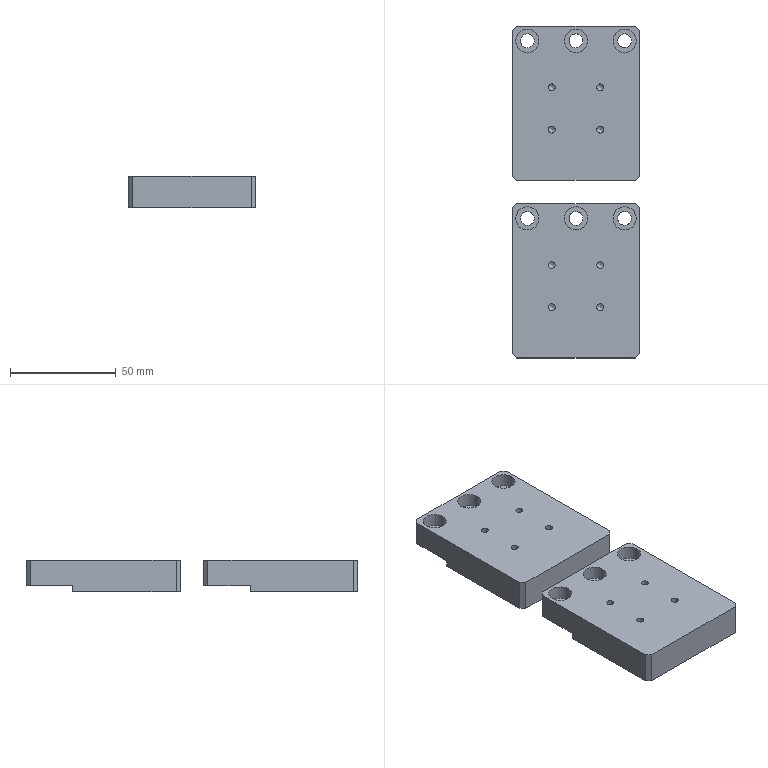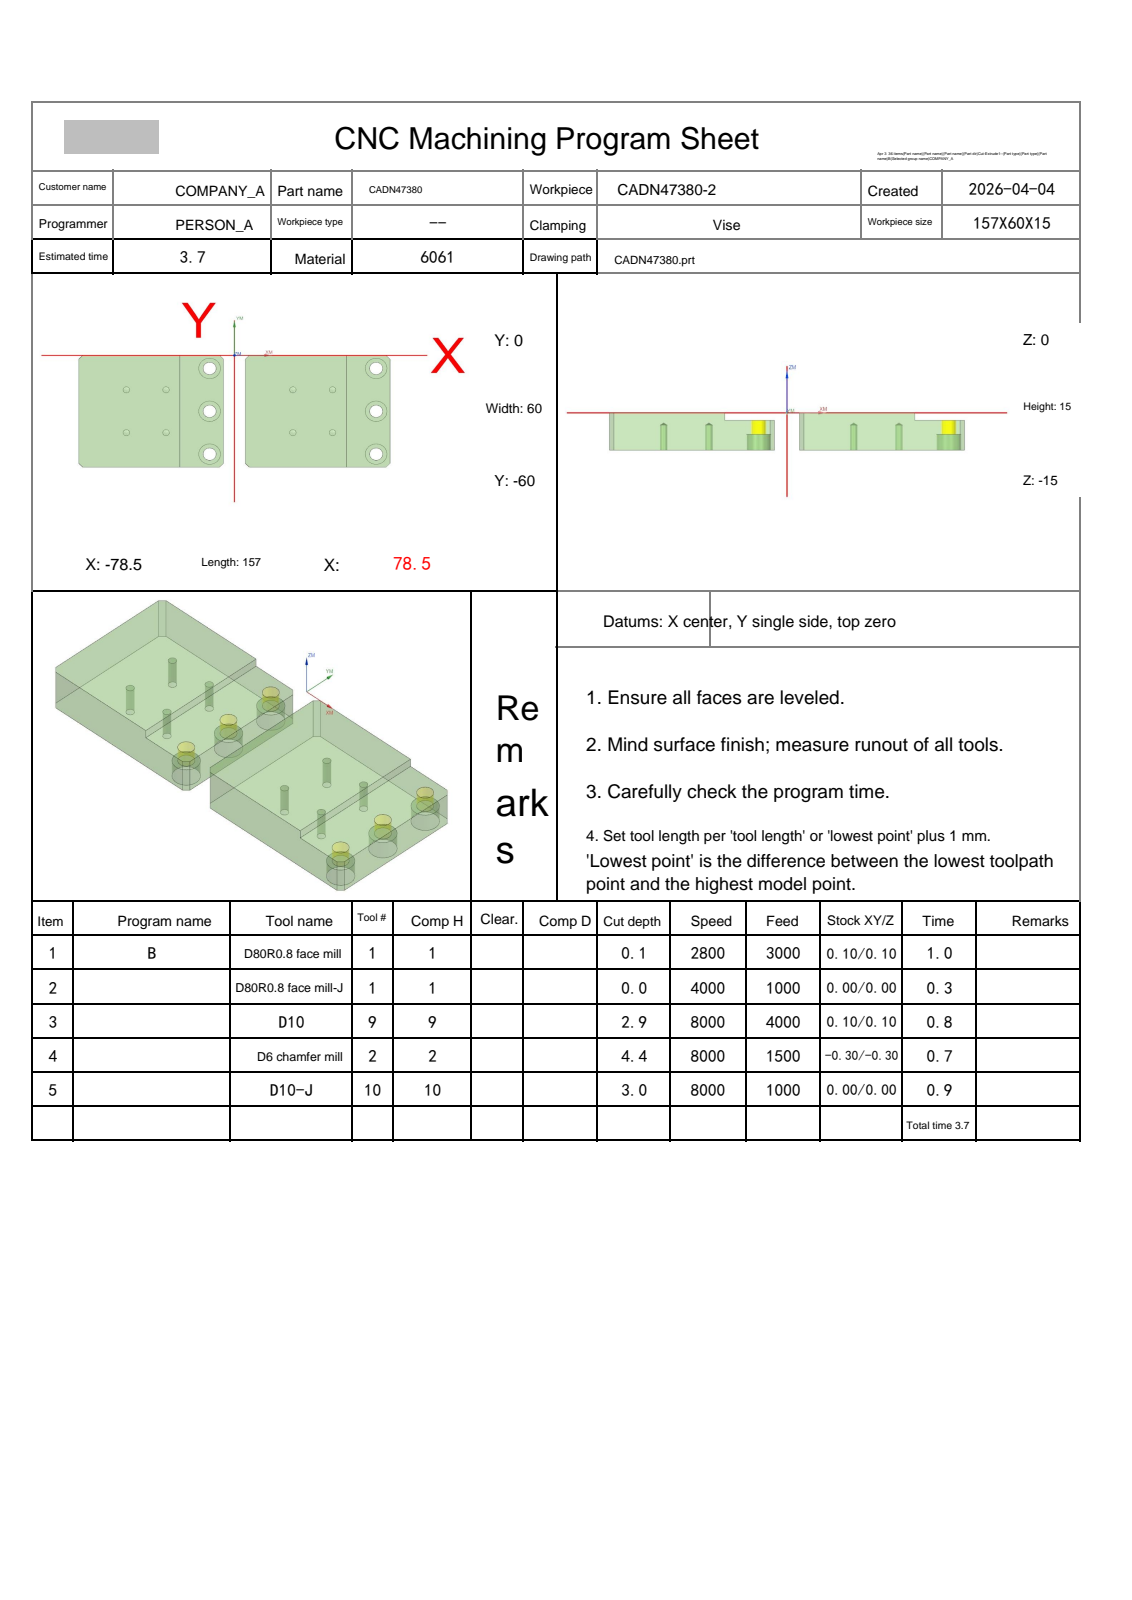NC program | NX | posted by the shop | part box 60 x 157 x 15 mm
Whole program:
%
O0001
(Machine time: 4.68 MIN)
(===Total Tool:4===)
(T1=D80R0.8 face mill D=80.  R=0.8  D-  H01 Z=0.    )
(T9=D10     D=10.  R=0.   D-  H09 Z=-2.9  )
(T2=D6 chamfer mill   D=6.   R=0.   D-  H02 Z=-4.4  )
(T10=D10-J  D=10.  R=0.   D10 H10 Z=-3.   )
G80 G90 G17 G49 G40
G91 G28 Z0
M01
N1 T01 M06
(D80R0.8 face mill  D=80. R=0.8 H=01 ce=0.10 di=0.10)
G00 G90 G54 X-130.597 Y-30. M03 S2800
G43 H01 Z20.
M08
Z6.011
G01 Z4.011 F3000.
X-118.597
X118.597
X130.597
Z6.011
G00 X-130.597
Z5.522
G01 Z3.522
X-118.597
X118.597
X130.597
Z5.522
G00 X-130.597
Z5.033
G01 Z3.033
X-118.597
X118.597
X130.597
Z5.033
G00 X-130.597
Z4.544
G01 Z2.544
X-118.597
X118.597
X130.597
Z4.544
G00 Z20.
X-130.597
Z4.056
G01 Z2.056
X-118.597
X118.597
X130.597
Z4.056
G00 Z20.
X-130.597
Z3.567
G01 Z1.567
X-118.597
X118.597
X130.597
Z3.567
G00 Z20.
X-130.597
Z3.078
G01 Z1.078
X-118.597
X118.597
X130.597
Z3.078
G00 Z20.
X-130.597
Z2.589
G01 Z.589
X-118.597
X118.597
X130.597
Z2.589
G00 Z20.
X-130.597
Z2.1
G01 Z.1
X-118.597
X118.597
X130.597
Z2.1
G00 Z20.
G91 G28 Z0.0
M05
M09
G91 G28 Z0.0
M01
N2 T01 M06
(D80R0.8 face mill-J  D=80. R=0.8 H=01 ce=0.00 di=0.00)
G00 G90 G54 X-130.499 Y-30. M03 S4000
G43 H01 Z20.
M08
Z2.
G01 Z0.0 F1000.
X-118.499
X118.499
X130.499
Z2.
G00 Z20.
G91 G28 Z0.0
M05
M09
G91 G28 Z0.0
M01
N3 T09 M06
(D10  D=10. R=0. H=09 ce=0.10 di=0.10)
G00 G90 G54 X-2.4 Y-66.214 M03 S8000
G43 H09 Z14.5
M08
Z.92
G01 Z-.58 F4000.
Y-61.83
Y1.416
G03 X-2.692 Y2.122 I-1. J-.001
G01 X-5.178 Y4.607
G03 X-5.884 Y4.9 I-.707 J-.707
G01 X-6.401
G03 X-7.4 Y3.901 I.001 J-1.
G01 Y-63.901
G02 X-8.399 Y-64.9 I-1. J.001
G01 X-13.901
G02 X-14.9 Y-63.901 I.001 J1.
G01 Y4.044
G03 X-15.746 Y5.032 I-1. J-.001
G01 X-21.246 Y5.888
X-21.4 Y5.9
G03 X-22.4 Y4.9 I0.0 J-1.
G01 Y-64.9
Y-68.1
Z.92
G00 X-2.4 Y-66.214
Z.34
G01 Z-1.16
Y-61.83
Y1.416
G03 X-2.692 Y2.122 I-1. J-.001
G01 X-5.178 Y4.607
G03 X-5.884 Y4.9 I-.707 J-.707
G01 X-6.401
G03 X-7.4 Y3.901 I.001 J-1.
G01 Y-63.901
G02 X-8.399 Y-64.9 I-1. J.001
G01 X-13.901
G02 X-14.9 Y-63.901 I.001 J1.
G01 Y4.044
G03 X-15.746 Y5.032 I-1. J-.001
G01 X-21.246 Y5.888
X-21.4 Y5.9
G03 X-22.4 Y4.9 I0.0 J-1.
G01 Y-64.9
Y-68.1
Z.34
G00 X-2.4 Y-66.214
Z-.24
G01 Z-1.74
Y-61.83
Y1.416
G03 X-2.692 Y2.122 I-1. J-.001
G01 X-5.178 Y4.607
G03 X-5.884 Y4.9 I-.707 J-.707
G01 X-6.401
G03 X-7.4 Y3.901 I.001 J-1.
G01 Y-63.901
G02 X-8.399 Y-64.9 I-1. J.001
G01 X-13.901
G02 X-14.9 Y-63.901 I.001 J1.
G01 Y4.044
G03 X-15.746 Y5.032 I-1. J-.001
G01 X-21.246 Y5.888
X-21.4 Y5.9
G03 X-22.4 Y4.9 I0.0 J-1.
G01 Y-64.9
Y-68.1
Z-.24
G00 X-2.4 Y-66.214
Z-.82
G01 Z-2.32
Y-61.83
Y1.416
G03 X-2.692 Y2.122 I-1. J-.001
G01 X-5.178 Y4.607
G03 X-5.884 Y4.9 I-.707 J-.707
G01 X-6.401
G03 X-7.4 Y3.901 I.001 J-1.
G01 Y-63.901
G02 X-8.399 Y-64.9 I-1. J.001
G01 X-13.901
G02 X-14.9 Y-63.901 I.001 J1.
G01 Y4.044
G03 X-15.746 Y5.032 I-1. J-.001
G01 X-21.246 Y5.888
X-21.4 Y5.9
G03 X-22.4 Y4.9 I0.0 J-1.
G01 Y-64.9
Y-68.1
Z-.82
G00 X-2.4 Y-66.214
Z-1.4
G01 Z-2.9
Y-61.83
Y1.416
G03 X-2.692 Y2.122 I-1. J-.001
G01 X-5.178 Y4.607
G03 X-5.884 Y4.9 I-.707 J-.707
G01 X-6.401
G03 X-7.4 Y3.901 I.001 J-1.
G01 Y-63.901
G02 X-8.399 Y-64.9 I-1. J.001
G01 X-13.901
G02 X-14.9 Y-63.901 I.001 J1.
G01 Y4.044
G03 X-15.746 Y5.032 I-1. J-.001
G01 X-21.246 Y5.888
X-21.4 Y5.9
G03 X-22.4 Y4.9 I0.0 J-1.
G01 Y-64.9
Y-68.1
Z-1.4
G00 Z3.
X81.6 Y-66.214
Z.92
G01 Z-.58
Y-61.83
Y1.416
G03 X81.308 Y2.122 I-1. J-.001
G01 X78.822 Y4.607
G03 X78.116 Y4.9 I-.707 J-.707
G01 X77.599
G03 X76.6 Y3.901 I.001 J-1.
G01 Y-63.901
G02 X75.601 Y-64.9 I-1. J.001
G01 X70.099
G02 X69.1 Y-63.901 I.001 J1.
G01 Y4.044
G03 X68.254 Y5.032 I-1. J-.001
G01 X62.754 Y5.888
X62.6 Y5.9
G03 X61.6 Y4.9 I0.0 J-1.
G01 Y-64.9
Y-68.1
Z.92
G00 X81.6 Y-66.214
Z.34
G01 Z-1.16
Y-61.83
Y1.416
G03 X81.308 Y2.122 I-1. J-.001
G01 X78.822 Y4.607
G03 X78.116 Y4.9 I-.707 J-.707
G01 X77.599
G03 X76.6 Y3.901 I.001 J-1.
G01 Y-63.901
G02 X75.601 Y-64.9 I-1. J.001
G01 X70.099
G02 X69.1 Y-63.901 I.001 J1.
G01 Y4.044
G03 X68.254 Y5.032 I-1. J-.001
G01 X62.754 Y5.888
X62.6 Y5.9
G03 X61.6 Y4.9 I0.0 J-1.
G01 Y-64.9
Y-68.1
Z.34
G00 X81.6 Y-66.214
Z-.24
G01 Z-1.74
Y-61.83
Y1.416
G03 X81.308 Y2.122 I-1. J-.001
G01 X78.822 Y4.607
G03 X78.116 Y4.9 I-.707 J-.707
G01 X77.599
G03 X76.6 Y3.901 I.001 J-1.
G01 Y-63.901
G02 X75.601 Y-64.9 I-1. J.001
G01 X70.099
G02 X69.1 Y-63.901 I.001 J1.
G01 Y4.044
G03 X68.254 Y5.032 I-1. J-.001
G01 X62.754 Y5.888
X62.6 Y5.9
G03 X61.6 Y4.9 I0.0 J-1.
G01 Y-64.9
Y-68.1
Z-.24
G00 X81.6 Y-66.214
Z-.82
G01 Z-2.32
Y-61.83
Y1.416
G03 X81.308 Y2.122 I-1. J-.001
G01 X78.822 Y4.607
G03 X78.116 Y4.9 I-.707 J-.707
G01 X77.599
G03 X76.6 Y3.901 I.001 J-1.
G01 Y-63.901
G02 X75.601 Y-64.9 I-1. J.001
G01 X70.099
G02 X69.1 Y-63.901 I.001 J1.
G01 Y4.044
G03 X68.254 Y5.032 I-1. J-.001
G01 X62.754 Y5.888
X62.6 Y5.9
G03 X61.6 Y4.9 I0.0 J-1.
G01 Y-64.9
Y-68.1
Z-.82
G00 X81.6 Y-66.214
Z-1.4
G01 Z-2.9
Y-61.83
Y1.416
G03 X81.308 Y2.122 I-1. J-.001
G01 X78.822 Y4.607
G03 X78.116 Y4.9 I-.707 J-.707
G01 X77.599
G03 X76.6 Y3.901 I.001 J-1.
G01 Y-63.901
G02 X75.601 Y-64.9 I-1. J.001
G01 X70.099
G02 X69.1 Y-63.901 I.001 J1.
G01 Y4.044
G03 X68.254 Y5.032 I-1. J-.001
G01 X62.754 Y5.888
X62.6 Y5.9
G03 X61.6 Y4.9 I0.0 J-1.
G01 Y-64.9
Y-68.1
Z-1.4
G00 Z14.5
G91 G28 Z0.0
M05
M09
G91 G28 Z0.0
M01
N4 T02 M06
(D6 chamfer mill  D=6. R=0. H=02 ce=-0.30 di=-0.80)
G00 G90 G54 X-11.413 Y-52.493 M03 S8000
G43 H02 Z20.
M08
Z-3.9
G01 Z-4.4 F1200.
X-11. Y-52.3
G03 X-12.5 Y-50.8 I-1.5 J0.0
X-14.7 Y-53. I0.0 J-2.2
X-12.5 Y-55.2 I2.2 J0.0
X-10.3 Y-53. I0.0 J2.2
X-12.5 Y-50.8 I-2.2 J0.0
X-14. Y-52.3 I0.0 J-1.5
G01 X-13.587 Y-52.493
Z-3.9
G00 Z20.
X-11.413 Y-29.493
Z-3.9
G01 Z-4.4
X-11. Y-29.3
G03 X-12.5 Y-27.8 I-1.5 J0.0
X-14.7 Y-30. I0.0 J-2.2
X-12.5 Y-32.2 I2.2 J0.0
X-10.3 Y-30. I0.0 J2.2
X-12.5 Y-27.8 I-2.2 J0.0
X-14. Y-29.3 I0.0 J-1.5
G01 X-13.587 Y-29.493
Z-3.9
G00 Z20.
X-11.413 Y-6.493
Z-3.9
G01 Z-4.4
X-11. Y-6.3
G03 X-12.5 Y-4.8 I-1.5 J0.0
X-14.7 Y-7. I0.0 J-2.2
X-12.5 Y-9.2 I2.2 J0.0
X-10.3 Y-7. I0.0 J2.2
X-12.5 Y-4.8 I-2.2 J0.0
X-14. Y-6.3 I0.0 J-1.5
G01 X-13.587 Y-6.493
Z-3.9
G00 Z20.
X72.587
Z-3.9
G01 Z-4.4
X73. Y-6.3
G03 X71.5 Y-4.8 I-1.5 J0.0
X69.3 Y-7. I0.0 J-2.2
X71.5 Y-9.2 I2.2 J0.0
X73.7 Y-7. I0.0 J2.2
X71.5 Y-4.8 I-2.2 J0.0
X70. Y-6.3 I0.0 J-1.5
G01 X70.413 Y-6.493
Z-3.9
G00 Z20.
X72.587 Y-29.493
Z-3.9
G01 Z-4.4
X73. Y-29.3
G03 X71.5 Y-27.8 I-1.5 J0.0
X69.3 Y-30. I0.0 J-2.2
X71.5 Y-32.2 I2.2 J0.0
X73.7 Y-30. I0.0 J2.2
X71.5 Y-27.8 I-2.2 J0.0
X70. Y-29.3 I0.0 J-1.5
G01 X70.413 Y-29.493
Z-3.9
G00 Z20.
X72.587 Y-52.493
Z-3.9
G01 Z-4.4
X73. Y-52.3
G03 X71.5 Y-50.8 I-1.5 J0.0
X69.3 Y-53. I0.0 J-2.2
X71.5 Y-55.2 I2.2 J0.0
X73.7 Y-53. I0.0 J2.2
X71.5 Y-50.8 I-2.2 J0.0
X70. Y-52.3 I0.0 J-1.5
G01 X70.413 Y-52.493
Z-3.9
G00 Z20.
G00 G90 X57.627 Y-29.614 M03 S8000
Z20.
Z.272
G01 Z-1.2 F1350.
G03 X57.427 Y-29.9 I1.532 J-1.286
G01 X57.397 Y-29.946
X57.4 Y-30.
Y-60. F1500.
G02 X56.5 Y-60.9 I-.9 J0.0
G01 X7.5
X7.267 Y-60.869
X7.05 Y-60.779
X6.864 Y-60.636
X4.864 Y-58.636
X4.721 Y-58.45
X4.631 Y-58.233
X4.6 Y-58.
Y-2.
X4.631 Y-1.767
X4.721 Y-1.55
X4.864 Y-1.364
X6.864 Y.636
X7.05 Y.779
X7.267 Y.869
X7.5 Y.9
X56.5
G02 X57.4 Y0.0 I0.0 J-.9
G01 Y-30.
X57.397 Y-30.054
X57.427 Y-30.1
G03 X57.627 Y-30.386 I1.732 J1.
G01 Z.272
G00 Z10.
X-26.373 Y-29.614
Z.272
G01 Z-1.2 F1350.
G03 X-26.573 Y-29.9 I1.532 J-1.286
G01 X-26.603 Y-29.946
X-26.6 Y-30.
Y-60. F1500.
G02 X-27.5 Y-60.9 I-.9 J0.0
G01 X-76.5
X-76.733 Y-60.869
X-76.95 Y-60.779
X-77.136 Y-60.636
X-79.136 Y-58.636
X-79.279 Y-58.45
X-79.369 Y-58.233
X-79.4 Y-58.
Y-2.
X-79.369 Y-1.767
X-79.279 Y-1.55
X-79.136 Y-1.364
X-77.136 Y.636
X-76.95 Y.779
X-76.733 Y.869
X-76.5 Y.9
X-27.5
G02 X-26.6 Y0.0 I0.0 J-.9
G01 Y-30.
X-26.603 Y-30.054
X-26.573 Y-30.1
G03 X-26.373 Y-30.386 I1.732 J1.
G01 Z.272
G00 Z10.
X-24.452 Y.968
Z-1.8
G01 Z-4.2 F1350.
X-24.366 Y.908
X-24.336 Y.9
X-7.5 F1500.
X-7.267 Y.869
X-7.05 Y.779
X-6.864 Y.636
X-4.864 Y-1.364
X-4.721 Y-1.55
X-4.631 Y-1.767
X-4.6 Y-2.
Y-58.
X-4.631 Y-58.233
X-4.721 Y-58.45
X-4.864 Y-58.636
X-6.864 Y-60.636
X-7.05 Y-60.779
X-7.267 Y-60.869
X-7.5 Y-60.9
X-24.336
X-24.366 Y-60.908
X-24.452 Y-60.968
Z-1.8
G00 Z10.
X-12.096 Y-4.792
Z-2.65
G01 Z-4.2 F1350.
G03 X-12.398 Y-4.618 I-1.147 J-1.638
G01 X-12.446 Y-4.592
X-12.5 Y-4.6
G03 X-14.9 Y-7. I0.0 J-2.4 F1500.
X-12.5 Y-9.4 I2.4 J0.0
X-10.1 Y-7. I0.0 J2.4
X-12.5 Y-4.6 I-2.4 J0.0
G01 X-12.554 Y-4.592
X-12.602 Y-4.618
G03 X-12.904 Y-4.792 I.845 J-1.813
G01 Z-2.65
G00 Z10.
X-12.096 Y-27.792
Z-2.65
G01 Z-4.2 F1350.
G03 X-12.398 Y-27.618 I-1.147 J-1.638
G01 X-12.446 Y-27.592
X-12.5 Y-27.6
G03 X-14.9 Y-30. I0.0 J-2.4 F1500.
X-12.5 Y-32.4 I2.4 J0.0
X-10.1 Y-30. I0.0 J2.4
X-12.5 Y-27.6 I-2.4 J0.0
G01 X-12.554 Y-27.592
X-12.602 Y-27.618
G03 X-12.904 Y-27.792 I.845 J-1.813
G01 Z-2.65
G00 Z10.
X-12.096 Y-50.792
Z-2.65
G01 Z-4.2 F1350.
G03 X-12.398 Y-50.618 I-1.147 J-1.638
G01 X-12.446 Y-50.592
X-12.5 Y-50.6
G03 X-14.9 Y-53. I0.0 J-2.4 F1500.
X-12.5 Y-55.4 I2.4 J0.0
X-10.1 Y-53. I0.0 J2.4
X-12.5 Y-50.6 I-2.4 J0.0
G01 X-12.554 Y-50.592
X-12.602 Y-50.618
G03 X-12.904 Y-50.792 I.845 J-1.813
G01 Z-2.65
G00 Z10.
X59.548 Y.968
Z-1.8
G01 Z-4.2 F1350.
X59.634 Y.908
X59.664 Y.9
X76.5 F1500.
X76.733 Y.869
X76.95 Y.779
X77.136 Y.636
X79.136 Y-1.364
X79.279 Y-1.55
X79.369 Y-1.767
X79.4 Y-2.
Y-58.
X79.369 Y-58.233
X79.279 Y-58.45
X79.136 Y-58.636
X77.136 Y-60.636
X76.95 Y-60.779
X76.733 Y-60.869
X76.5 Y-60.9
X59.664
X59.634 Y-60.908
X59.548 Y-60.968
Z-1.8
G00 Z10.
X71.904 Y-4.792
Z-2.65
G01 Z-4.2 F1350.
G03 X71.602 Y-4.618 I-1.147 J-1.638
G01 X71.554 Y-4.592
X71.5 Y-4.6
G03 X69.1 Y-7. I0.0 J-2.4 F1500.
X71.5 Y-9.4 I2.4 J0.0
X73.9 Y-7. I0.0 J2.4
X71.5 Y-4.6 I-2.4 J0.0
G01 X71.446 Y-4.592
X71.398 Y-4.618
G03 X71.096 Y-4.792 I.845 J-1.813
G01 Z-2.65
G00 Z10.
X71.904 Y-27.792
Z-2.65
G01 Z-4.2 F1350.
G03 X71.602 Y-27.618 I-1.147 J-1.638
G01 X71.554 Y-27.592
X71.5 Y-27.6
G03 X69.1 Y-30. I0.0 J-2.4 F1500.
X71.5 Y-32.4 I2.4 J0.0
X73.9 Y-30. I0.0 J2.4
X71.5 Y-27.6 I-2.4 J0.0
G01 X71.446 Y-27.592
X71.398 Y-27.618
G03 X71.096 Y-27.792 I.845 J-1.813
G01 Z-2.65
G00 Z10.
X71.904 Y-50.792
Z-2.65
G01 Z-4.2 F1350.
G03 X71.602 Y-50.618 I-1.147 J-1.638
G01 X71.554 Y-50.592
X71.5 Y-50.6
G03 X69.1 Y-53. I0.0 J-2.4 F1500.
X71.5 Y-55.4 I2.4 J0.0
X73.9 Y-53. I0.0 J2.4
X71.5 Y-50.6 I-2.4 J0.0
G01 X71.446 Y-50.592
X71.398 Y-50.618
G03 X71.096 Y-50.792 I.845 J-1.813
G01 Z-2.65
G00 Z20.
G91 G28 Z0.0
M05
M09
G91 G28 Z0.0
M01
N5 T10 M06
(D10-J  D=10. R=0. H=10 ce=0.40 di=0.00)
G00 G90 G54 X-3.438 Y5.837 M03 S8000
G43 H10 Z14.5
M08
Z-1.5
G01 Z-3. F1000.
G03 X-4.5 Y4.071 I.938 J-1.766
G01 Y-63.657
G02 X-4.793 Y-64.364 I-1. J.001
G01 X-5.136 Y-64.707
G02 X-5.843 Y-65. I-.707 J.707
G01 X-7.901
G02 X-8.9 Y-64.001 I.001 J1.
G01 Y4.1
G03 X-9.8 Y5. I-.9 J0.0
G01 X-12.3
G03 X-13.3 Y4. I0.0 J-1.
G01 Y-64.
G02 X-14.3 Y-65. I-1. J0.0
G01 X-16.8
G02 X-17.7 Y-64.1 I0.0 J.9
G01 Y4.1
G03 X-18.6 Y5. I-.9 J0.0
G01 X-21.1
G03 X-22.1 Y4. I0.0 J-1.
G01 Y-65.
G03 X-20.1 Y-67. I2. J0.0
G01 Z-1.5
G00 Z14.5
X80.562 Y5.837
Z-1.5
G01 Z-3.
G03 X79.5 Y4.071 I.938 J-1.766
G01 Y-63.657
G02 X79.208 Y-64.364 I-1. J.001
G01 X78.864 Y-64.707
G02 X78.157 Y-65. I-.707 J.707
G01 X76.099
G02 X75.1 Y-64.001 I.001 J1.
G01 Y4.1
G03 X74.2 Y5. I-.9 J0.0
G01 X71.7
G03 X70.7 Y4. I0.0 J-1.
G01 Y-64.1
G02 X69.8 Y-65. I-.9 J0.0
G01 X67.3
G02 X66.3 Y-64. I0.0 J1.
G01 Y4.1
G03 X65.4 Y5. I-.9 J0.0
G01 X62.9
G03 X61.9 Y4. I0.0 J-1.
G01 Y-65.
G03 X63.9 Y-67. I2. J0.0
G01 Z-1.5
G00 Z14.5
G00 G90 X-20.301 Y7. M03 S8000
Z14.5
Z-2.
G01 Z-3. F1000.
G41 D10
X-20.501
G03 X-22.5 Y5. I.001 J-2.
G01 Y-65.
G03 X-20.501 Y-67. I2. J0.0
G01 G40 X-20.301
Z-2.
G00 Z14.5
X63.699 Y7.
Z-2.
G01 Z-3.
G41 D10
X63.499
G03 X61.5 Y5. I.001 J-2.
G01 Y-65.
G03 X63.499 Y-67. I2. J0.0
G01 G40 X63.699
Z-2.
G00 Z14.5
M05
M09
G91 G28 Z0.0
G91 G28 Y0.0
M30
%